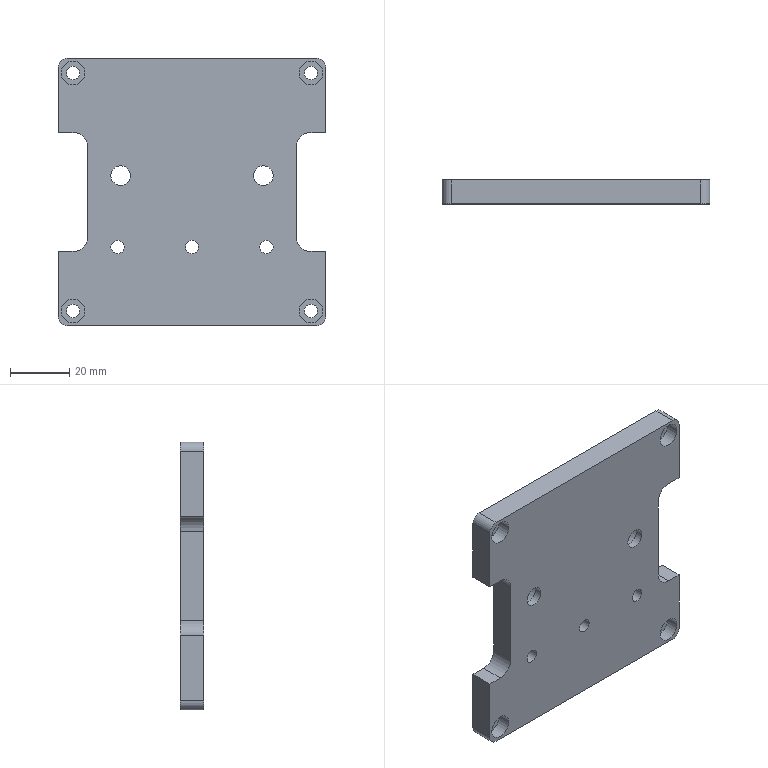Part | NX | 1 solid | 53 faces | box 90 x 8 x 90 mm | volume 55259 mm3 | cylinder 28 | plane 23 | cone 2 | commonest cylinder face diameters 4.5 x7 8 x7 6 x4 10 x4 2.5 x2 6.6 x2
STEP:
#1=CARTESIAN_POINT('',(45.,-4.,42.));
#2=VERTEX_POINT('',#1);
#3=CARTESIAN_POINT('',(45.,-4.,20.));
#4=VERTEX_POINT('',#3);
#5=CARTESIAN_POINT('',(45.,-4.,45.));
#6=DIRECTION('',(0.,0.,-1.));
#7=VECTOR('',#6,1000.);
#8=LINE('',#5,#7);
#9=EDGE_CURVE('',#2,#4,#8,.T.);
#10=ORIENTED_EDGE('',*,*,#9,.T.);
#11=CARTESIAN_POINT('',(45.,4.,20.));
#12=VERTEX_POINT('',#11);
#13=CARTESIAN_POINT('',(45.,4.,20.));
#14=DIRECTION('',(0.,1.,0.));
#15=VECTOR('',#14,1000.);
#16=LINE('',#13,#15);
#17=EDGE_CURVE('',#4,#12,#16,.T.);
#18=ORIENTED_EDGE('',*,*,#17,.T.);
#19=CARTESIAN_POINT('',(45.,4.,42.));
#20=VERTEX_POINT('',#19);
#21=CARTESIAN_POINT('',(45.,4.,45.));
#22=DIRECTION('',(0.,0.,-1.));
#23=VECTOR('',#22,1000.);
#24=LINE('',#21,#23);
#25=EDGE_CURVE('',#20,#12,#24,.T.);
#26=ORIENTED_EDGE('',*,*,#25,.F.);
#27=CARTESIAN_POINT('',(45.,4.,42.));
#28=DIRECTION('',(0.,-1.,0.));
#29=VECTOR('',#28,1000.);
#30=LINE('',#27,#29);
#31=EDGE_CURVE('',#20,#2,#30,.T.);
#32=ORIENTED_EDGE('',*,*,#31,.T.);
#33=EDGE_LOOP('',(#10,#18,#26,#32));
#34=FACE_BOUND('',#33,.T.);
#35=CARTESIAN_POINT('',(45.,4.,45.));
#36=DIRECTION('',(-1.,0.,0.));
#37=DIRECTION('',(0.,0.,1.));
#38=AXIS2_PLACEMENT_3D('',#35,#36,#37);
#39=PLANE('',#38);
#40=ADVANCED_FACE('',(#34),#39,.F.);
#41=CARTESIAN_POINT('',(-45.,4.,20.));
#42=VERTEX_POINT('',#41);
#43=CARTESIAN_POINT('',(-45.,4.,42.));
#44=VERTEX_POINT('',#43);
#45=CARTESIAN_POINT('',(-45.,4.,45.));
#46=DIRECTION('',(0.,0.,1.));
#47=VECTOR('',#46,1000.);
#48=LINE('',#45,#47);
#49=EDGE_CURVE('',#42,#44,#48,.T.);
#50=ORIENTED_EDGE('',*,*,#49,.F.);
#51=CARTESIAN_POINT('',(-45.,-4.,20.));
#52=VERTEX_POINT('',#51);
#53=CARTESIAN_POINT('',(-45.,4.,20.));
#54=DIRECTION('',(0.,-1.,0.));
#55=VECTOR('',#54,1000.);
#56=LINE('',#53,#55);
#57=EDGE_CURVE('',#42,#52,#56,.T.);
#58=ORIENTED_EDGE('',*,*,#57,.T.);
#59=CARTESIAN_POINT('',(-45.,-4.,42.));
#60=VERTEX_POINT('',#59);
#61=CARTESIAN_POINT('',(-45.,-4.,45.));
#62=DIRECTION('',(0.,0.,1.));
#63=VECTOR('',#62,1000.);
#64=LINE('',#61,#63);
#65=EDGE_CURVE('',#52,#60,#64,.T.);
#66=ORIENTED_EDGE('',*,*,#65,.T.);
#67=CARTESIAN_POINT('',(-45.,4.,42.));
#68=DIRECTION('',(0.,-1.,0.));
#69=VECTOR('',#68,1000.);
#70=LINE('',#67,#69);
#71=EDGE_CURVE('',#60,#44,#70,.F.);
#72=ORIENTED_EDGE('',*,*,#71,.T.);
#73=EDGE_LOOP('',(#50,#58,#66,#72));
#74=FACE_BOUND('',#73,.T.);
#75=CARTESIAN_POINT('',(-45.,4.,45.));
#76=DIRECTION('',(1.,0.,0.));
#77=DIRECTION('',(0.,0.,-1.));
#78=AXIS2_PLACEMENT_3D('',#75,#76,#77);
#79=PLANE('',#78);
#80=ADVANCED_FACE('',(#74),#79,.F.);
#81=CARTESIAN_POINT('',(-45.,-4.,-42.));
#82=VERTEX_POINT('',#81);
#83=CARTESIAN_POINT('',(-45.,-4.,-20.));
#84=VERTEX_POINT('',#83);
#85=CARTESIAN_POINT('',(-45.,-4.,45.));
#86=DIRECTION('',(0.,0.,1.));
#87=VECTOR('',#86,1000.);
#88=LINE('',#85,#87);
#89=EDGE_CURVE('',#82,#84,#88,.T.);
#90=ORIENTED_EDGE('',*,*,#89,.T.);
#91=CARTESIAN_POINT('',(-45.,4.,-20.));
#92=VERTEX_POINT('',#91);
#93=CARTESIAN_POINT('',(-45.,4.,-20.));
#94=DIRECTION('',(0.,1.,0.));
#95=VECTOR('',#94,1000.);
#96=LINE('',#93,#95);
#97=EDGE_CURVE('',#84,#92,#96,.T.);
#98=ORIENTED_EDGE('',*,*,#97,.T.);
#99=CARTESIAN_POINT('',(-45.,4.,-42.));
#100=VERTEX_POINT('',#99);
#101=CARTESIAN_POINT('',(-45.,4.,45.));
#102=DIRECTION('',(0.,0.,1.));
#103=VECTOR('',#102,1000.);
#104=LINE('',#101,#103);
#105=EDGE_CURVE('',#100,#92,#104,.T.);
#106=ORIENTED_EDGE('',*,*,#105,.F.);
#107=CARTESIAN_POINT('',(-45.,4.,-42.));
#108=DIRECTION('',(0.,-1.,0.));
#109=VECTOR('',#108,1000.);
#110=LINE('',#107,#109);
#111=EDGE_CURVE('',#100,#82,#110,.T.);
#112=ORIENTED_EDGE('',*,*,#111,.T.);
#113=EDGE_LOOP('',(#90,#98,#106,#112));
#114=FACE_BOUND('',#113,.T.);
#115=CARTESIAN_POINT('',(-45.,4.,45.));
#116=DIRECTION('',(1.,0.,0.));
#117=DIRECTION('',(0.,0.,-1.));
#118=AXIS2_PLACEMENT_3D('',#115,#116,#117);
#119=PLANE('',#118);
#120=ADVANCED_FACE('',(#114),#119,.F.);
#121=CARTESIAN_POINT('',(-42.,-4.,45.));
#122=VERTEX_POINT('',#121);
#123=CARTESIAN_POINT('',(42.,-4.,45.));
#124=VERTEX_POINT('',#123);
#125=CARTESIAN_POINT('',(45.,-4.,45.));
#126=DIRECTION('',(1.,0.,0.));
#127=VECTOR('',#126,1000.);
#128=LINE('',#125,#127);
#129=EDGE_CURVE('',#122,#124,#128,.T.);
#130=ORIENTED_EDGE('',*,*,#129,.T.);
#131=CARTESIAN_POINT('',(42.,4.,45.));
#132=VERTEX_POINT('',#131);
#133=CARTESIAN_POINT('',(42.,4.,45.));
#134=DIRECTION('',(0.,-1.,0.));
#135=VECTOR('',#134,1000.);
#136=LINE('',#133,#135);
#137=EDGE_CURVE('',#124,#132,#136,.F.);
#138=ORIENTED_EDGE('',*,*,#137,.T.);
#139=CARTESIAN_POINT('',(-42.,4.,45.));
#140=VERTEX_POINT('',#139);
#141=CARTESIAN_POINT('',(45.,4.,45.));
#142=DIRECTION('',(1.,0.,0.));
#143=VECTOR('',#142,1000.);
#144=LINE('',#141,#143);
#145=EDGE_CURVE('',#140,#132,#144,.T.);
#146=ORIENTED_EDGE('',*,*,#145,.F.);
#147=CARTESIAN_POINT('',(-42.,4.,45.));
#148=DIRECTION('',(0.,-1.,0.));
#149=VECTOR('',#148,1000.);
#150=LINE('',#147,#149);
#151=EDGE_CURVE('',#140,#122,#150,.T.);
#152=ORIENTED_EDGE('',*,*,#151,.T.);
#153=EDGE_LOOP('',(#130,#138,#146,#152));
#154=FACE_BOUND('',#153,.T.);
#155=CARTESIAN_POINT('',(45.,4.,45.));
#156=DIRECTION('',(0.,0.,-1.));
#157=DIRECTION('',(-1.,0.,0.));
#158=AXIS2_PLACEMENT_3D('',#155,#156,#157);
#159=PLANE('',#158);
#160=ADVANCED_FACE('',(#154),#159,.F.);
#161=CARTESIAN_POINT('',(45.,4.,-20.));
#162=VERTEX_POINT('',#161);
#163=CARTESIAN_POINT('',(45.,4.,-42.));
#164=VERTEX_POINT('',#163);
#165=CARTESIAN_POINT('',(45.,4.,45.));
#166=DIRECTION('',(0.,0.,-1.));
#167=VECTOR('',#166,1000.);
#168=LINE('',#165,#167);
#169=EDGE_CURVE('',#162,#164,#168,.T.);
#170=ORIENTED_EDGE('',*,*,#169,.F.);
#171=CARTESIAN_POINT('',(45.,-4.,-20.));
#172=VERTEX_POINT('',#171);
#173=CARTESIAN_POINT('',(45.,4.,-20.));
#174=DIRECTION('',(0.,-1.,0.));
#175=VECTOR('',#174,1000.);
#176=LINE('',#173,#175);
#177=EDGE_CURVE('',#162,#172,#176,.T.);
#178=ORIENTED_EDGE('',*,*,#177,.T.);
#179=CARTESIAN_POINT('',(45.,-4.,-42.));
#180=VERTEX_POINT('',#179);
#181=CARTESIAN_POINT('',(45.,-4.,45.));
#182=DIRECTION('',(0.,0.,-1.));
#183=VECTOR('',#182,1000.);
#184=LINE('',#181,#183);
#185=EDGE_CURVE('',#172,#180,#184,.T.);
#186=ORIENTED_EDGE('',*,*,#185,.T.);
#187=CARTESIAN_POINT('',(45.,4.,-42.));
#188=DIRECTION('',(0.,-1.,0.));
#189=VECTOR('',#188,1000.);
#190=LINE('',#187,#189);
#191=EDGE_CURVE('',#180,#164,#190,.F.);
#192=ORIENTED_EDGE('',*,*,#191,.T.);
#193=EDGE_LOOP('',(#170,#178,#186,#192));
#194=FACE_BOUND('',#193,.T.);
#195=CARTESIAN_POINT('',(45.,4.,45.));
#196=DIRECTION('',(-1.,0.,0.));
#197=DIRECTION('',(0.,0.,1.));
#198=AXIS2_PLACEMENT_3D('',#195,#196,#197);
#199=PLANE('',#198);
#200=ADVANCED_FACE('',(#194),#199,.F.);
#201=CARTESIAN_POINT('',(-13.75,0.,-45.));
#202=VERTEX_POINT('',#201);
#203=CARTESIAN_POINT('',(-12.5,0.,-45.));
#204=DIRECTION('',(0.,0.,-1.));
#205=DIRECTION('',(-1.,0.,0.));
#206=AXIS2_PLACEMENT_3D('',#203,#204,#205);
#207=CIRCLE('',#206,1.25);
#208=EDGE_CURVE('',#202,#202,#207,.T.);
#209=ORIENTED_EDGE('',*,*,#208,.F.);
#210=EDGE_LOOP('',(#209));
#211=FACE_BOUND('',#210,.T.);
#212=CARTESIAN_POINT('',(11.25,0.,-45.));
#213=VERTEX_POINT('',#212);
#214=CARTESIAN_POINT('',(12.5,0.,-45.));
#215=DIRECTION('',(0.,0.,-1.));
#216=DIRECTION('',(-1.,0.,0.));
#217=AXIS2_PLACEMENT_3D('',#214,#215,#216);
#218=CIRCLE('',#217,1.25);
#219=EDGE_CURVE('',#213,#213,#218,.T.);
#220=ORIENTED_EDGE('',*,*,#219,.F.);
#221=EDGE_LOOP('',(#220));
#222=FACE_BOUND('',#221,.T.);
#223=CARTESIAN_POINT('',(42.,-4.,-45.));
#224=VERTEX_POINT('',#223);
#225=CARTESIAN_POINT('',(-42.,-4.,-45.));
#226=VERTEX_POINT('',#225);
#227=CARTESIAN_POINT('',(45.,-4.,-45.));
#228=DIRECTION('',(-1.,0.,0.));
#229=VECTOR('',#228,1000.);
#230=LINE('',#227,#229);
#231=EDGE_CURVE('',#224,#226,#230,.T.);
#232=ORIENTED_EDGE('',*,*,#231,.T.);
#233=CARTESIAN_POINT('',(-42.,4.,-45.));
#234=VERTEX_POINT('',#233);
#235=CARTESIAN_POINT('',(-42.,4.,-45.));
#236=DIRECTION('',(0.,-1.,0.));
#237=VECTOR('',#236,1000.);
#238=LINE('',#235,#237);
#239=EDGE_CURVE('',#226,#234,#238,.F.);
#240=ORIENTED_EDGE('',*,*,#239,.T.);
#241=CARTESIAN_POINT('',(42.,4.,-45.));
#242=VERTEX_POINT('',#241);
#243=CARTESIAN_POINT('',(45.,4.,-45.));
#244=DIRECTION('',(-1.,0.,0.));
#245=VECTOR('',#244,1000.);
#246=LINE('',#243,#245);
#247=EDGE_CURVE('',#242,#234,#246,.T.);
#248=ORIENTED_EDGE('',*,*,#247,.F.);
#249=CARTESIAN_POINT('',(42.,4.,-45.));
#250=DIRECTION('',(0.,-1.,0.));
#251=VECTOR('',#250,1000.);
#252=LINE('',#249,#251);
#253=EDGE_CURVE('',#242,#224,#252,.T.);
#254=ORIENTED_EDGE('',*,*,#253,.T.);
#255=EDGE_LOOP('',(#232,#240,#248,#254));
#256=FACE_BOUND('',#255,.T.);
#257=CARTESIAN_POINT('',(45.,4.,-45.));
#258=DIRECTION('',(0.,0.,1.));
#259=DIRECTION('',(1.,0.,0.));
#260=AXIS2_PLACEMENT_3D('',#257,#258,#259);
#261=PLANE('',#260);
#262=ADVANCED_FACE('',(#211,#222,#256),#261,.F.);
#263=CARTESIAN_POINT('',(40.,4.,20.));
#264=VERTEX_POINT('',#263);
#265=CARTESIAN_POINT('',(35.,4.,20.));
#266=DIRECTION('',(-1.,0.,0.));
#267=VECTOR('',#266,1000.);
#268=LINE('',#265,#267);
#269=EDGE_CURVE('',#12,#264,#268,.T.);
#270=ORIENTED_EDGE('',*,*,#269,.T.);
#271=CARTESIAN_POINT('',(35.,4.,15.));
#272=VERTEX_POINT('',#271);
#273=CARTESIAN_POINT('',(40.,4.,15.));
#274=DIRECTION('',(0.,1.,0.));
#275=DIRECTION('',(0.,0.,1.));
#276=AXIS2_PLACEMENT_3D('',#273,#274,#275);
#277=CIRCLE('',#276,5.);
#278=EDGE_CURVE('',#264,#272,#277,.F.);
#279=ORIENTED_EDGE('',*,*,#278,.T.);
#280=CARTESIAN_POINT('',(35.,4.,-15.));
#281=VERTEX_POINT('',#280);
#282=CARTESIAN_POINT('',(35.,4.,20.));
#283=DIRECTION('',(0.,0.,-1.));
#284=VECTOR('',#283,1000.);
#285=LINE('',#282,#284);
#286=EDGE_CURVE('',#272,#281,#285,.T.);
#287=ORIENTED_EDGE('',*,*,#286,.T.);
#288=CARTESIAN_POINT('',(40.,4.,-20.));
#289=VERTEX_POINT('',#288);
#290=CARTESIAN_POINT('',(40.,4.,-15.));
#291=DIRECTION('',(0.,1.,0.));
#292=DIRECTION('',(0.,0.,1.));
#293=AXIS2_PLACEMENT_3D('',#290,#291,#292);
#294=CIRCLE('',#293,5.);
#295=EDGE_CURVE('',#281,#289,#294,.F.);
#296=ORIENTED_EDGE('',*,*,#295,.T.);
#297=CARTESIAN_POINT('',(35.,4.,-20.));
#298=DIRECTION('',(1.,0.,0.));
#299=VECTOR('',#298,1000.);
#300=LINE('',#297,#299);
#301=EDGE_CURVE('',#289,#162,#300,.T.);
#302=ORIENTED_EDGE('',*,*,#301,.T.);
#303=ORIENTED_EDGE('',*,*,#169,.T.);
#304=CARTESIAN_POINT('',(42.,4.,-42.));
#305=DIRECTION('',(0.,1.,0.));
#306=DIRECTION('',(0.,0.,1.));
#307=AXIS2_PLACEMENT_3D('',#304,#305,#306);
#308=CIRCLE('',#307,3.);
#309=EDGE_CURVE('',#164,#242,#308,.T.);
#310=ORIENTED_EDGE('',*,*,#309,.T.);
#311=ORIENTED_EDGE('',*,*,#247,.T.);
#312=CARTESIAN_POINT('',(-42.,4.,-42.));
#313=DIRECTION('',(0.,1.,0.));
#314=DIRECTION('',(0.,0.,1.));
#315=AXIS2_PLACEMENT_3D('',#312,#313,#314);
#316=CIRCLE('',#315,3.);
#317=EDGE_CURVE('',#234,#100,#316,.T.);
#318=ORIENTED_EDGE('',*,*,#317,.T.);
#319=ORIENTED_EDGE('',*,*,#105,.T.);
#320=CARTESIAN_POINT('',(-40.,4.,-20.));
#321=VERTEX_POINT('',#320);
#322=CARTESIAN_POINT('',(-35.,4.,-20.));
#323=DIRECTION('',(1.,0.,0.));
#324=VECTOR('',#323,1000.);
#325=LINE('',#322,#324);
#326=EDGE_CURVE('',#92,#321,#325,.T.);
#327=ORIENTED_EDGE('',*,*,#326,.T.);
#328=CARTESIAN_POINT('',(-35.,4.,-15.));
#329=VERTEX_POINT('',#328);
#330=CARTESIAN_POINT('',(-40.,4.,-15.));
#331=DIRECTION('',(0.,1.,0.));
#332=DIRECTION('',(0.,0.,1.));
#333=AXIS2_PLACEMENT_3D('',#330,#331,#332);
#334=CIRCLE('',#333,5.);
#335=EDGE_CURVE('',#321,#329,#334,.F.);
#336=ORIENTED_EDGE('',*,*,#335,.T.);
#337=CARTESIAN_POINT('',(-35.,4.,15.));
#338=VERTEX_POINT('',#337);
#339=CARTESIAN_POINT('',(-35.,4.,20.));
#340=DIRECTION('',(0.,0.,1.));
#341=VECTOR('',#340,1000.);
#342=LINE('',#339,#341);
#343=EDGE_CURVE('',#329,#338,#342,.T.);
#344=ORIENTED_EDGE('',*,*,#343,.T.);
#345=CARTESIAN_POINT('',(-40.,4.,20.));
#346=VERTEX_POINT('',#345);
#347=CARTESIAN_POINT('',(-40.,4.,15.));
#348=DIRECTION('',(0.,1.,0.));
#349=DIRECTION('',(0.,0.,1.));
#350=AXIS2_PLACEMENT_3D('',#347,#348,#349);
#351=CIRCLE('',#350,5.);
#352=EDGE_CURVE('',#338,#346,#351,.F.);
#353=ORIENTED_EDGE('',*,*,#352,.T.);
#354=CARTESIAN_POINT('',(-35.,4.,20.));
#355=DIRECTION('',(-1.,0.,0.));
#356=VECTOR('',#355,1000.);
#357=LINE('',#354,#356);
#358=EDGE_CURVE('',#346,#42,#357,.T.);
#359=ORIENTED_EDGE('',*,*,#358,.T.);
#360=ORIENTED_EDGE('',*,*,#49,.T.);
#361=CARTESIAN_POINT('',(-42.,4.,42.));
#362=DIRECTION('',(0.,1.,0.));
#363=DIRECTION('',(0.,0.,1.));
#364=AXIS2_PLACEMENT_3D('',#361,#362,#363);
#365=CIRCLE('',#364,3.);
#366=EDGE_CURVE('',#44,#140,#365,.T.);
#367=ORIENTED_EDGE('',*,*,#366,.T.);
#368=ORIENTED_EDGE('',*,*,#145,.T.);
#369=CARTESIAN_POINT('',(42.,4.,42.));
#370=DIRECTION('',(0.,1.,0.));
#371=DIRECTION('',(0.,0.,1.));
#372=AXIS2_PLACEMENT_3D('',#369,#370,#371);
#373=CIRCLE('',#372,3.);
#374=EDGE_CURVE('',#132,#20,#373,.T.);
#375=ORIENTED_EDGE('',*,*,#374,.T.);
#376=ORIENTED_EDGE('',*,*,#25,.T.);
#377=EDGE_LOOP('',(#270,#279,#287,#296,#302,#303,#310,#311,#318,#319,#327,#336,#344,#353,#359,#360,#367,#368,#375,#376));
#378=FACE_BOUND('',#377,.T.);
#379=CARTESIAN_POINT('',(-25.,4.,-14.5));
#380=VERTEX_POINT('',#379);
#381=CARTESIAN_POINT('',(-25.,4.,-18.5));
#382=DIRECTION('',(0.,1.,0.));
#383=DIRECTION('',(0.,0.,1.));
#384=AXIS2_PLACEMENT_3D('',#381,#382,#383);
#385=CIRCLE('',#384,4.);
#386=EDGE_CURVE('',#380,#380,#385,.T.);
#387=ORIENTED_EDGE('',*,*,#386,.F.);
#388=EDGE_LOOP('',(#387));
#389=FACE_BOUND('',#388,.T.);
#390=CARTESIAN_POINT('',(0.,4.,-14.5));
#391=VERTEX_POINT('',#390);
#392=CARTESIAN_POINT('',(0.,4.,-18.5));
#393=DIRECTION('',(0.,1.,0.));
#394=DIRECTION('',(0.,0.,1.));
#395=AXIS2_PLACEMENT_3D('',#392,#393,#394);
#396=CIRCLE('',#395,4.);
#397=EDGE_CURVE('',#391,#391,#396,.T.);
#398=ORIENTED_EDGE('',*,*,#397,.F.);
#399=EDGE_LOOP('',(#398));
#400=FACE_BOUND('',#399,.T.);
#401=CARTESIAN_POINT('',(25.,4.,-14.5));
#402=VERTEX_POINT('',#401);
#403=CARTESIAN_POINT('',(25.,4.,-18.5));
#404=DIRECTION('',(0.,1.,0.));
#405=DIRECTION('',(0.,0.,1.));
#406=AXIS2_PLACEMENT_3D('',#403,#404,#405);
#407=CIRCLE('',#406,4.);
#408=EDGE_CURVE('',#402,#402,#407,.T.);
#409=ORIENTED_EDGE('',*,*,#408,.F.);
#410=EDGE_LOOP('',(#409));
#411=FACE_BOUND('',#410,.T.);
#412=CARTESIAN_POINT('',(24.,4.,11.));
#413=VERTEX_POINT('',#412);
#414=CARTESIAN_POINT('',(24.,4.,5.5));
#415=DIRECTION('',(0.,1.,0.));
#416=DIRECTION('',(0.,0.,1.));
#417=AXIS2_PLACEMENT_3D('',#414,#415,#416);
#418=CIRCLE('',#417,5.5);
#419=EDGE_CURVE('',#413,#413,#418,.T.);
#420=ORIENTED_EDGE('',*,*,#419,.F.);
#421=EDGE_LOOP('',(#420));
#422=FACE_BOUND('',#421,.T.);
#423=CARTESIAN_POINT('',(-24.,4.,11.));
#424=VERTEX_POINT('',#423);
#425=CARTESIAN_POINT('',(-24.,4.,5.5));
#426=DIRECTION('',(0.,1.,0.));
#427=DIRECTION('',(0.,0.,1.));
#428=AXIS2_PLACEMENT_3D('',#425,#426,#427);
#429=CIRCLE('',#428,5.5);
#430=EDGE_CURVE('',#424,#424,#429,.T.);
#431=ORIENTED_EDGE('',*,*,#430,.F.);
#432=EDGE_LOOP('',(#431));
#433=FACE_BOUND('',#432,.T.);
#434=CARTESIAN_POINT('',(-40.,4.,-42.25));
#435=VERTEX_POINT('',#434);
#436=CARTESIAN_POINT('',(-40.,4.,-40.));
#437=DIRECTION('',(0.,-1.,0.));
#438=DIRECTION('',(0.,0.,-1.));
#439=AXIS2_PLACEMENT_3D('',#436,#437,#438);
#440=CIRCLE('',#439,2.25);
#441=EDGE_CURVE('',#435,#435,#440,.T.);
#442=ORIENTED_EDGE('',*,*,#441,.T.);
#443=EDGE_LOOP('',(#442));
#444=FACE_BOUND('',#443,.T.);
#445=CARTESIAN_POINT('',(40.,4.,-42.25));
#446=VERTEX_POINT('',#445);
#447=CARTESIAN_POINT('',(40.,4.,-40.));
#448=DIRECTION('',(0.,-1.,0.));
#449=DIRECTION('',(0.,0.,-1.));
#450=AXIS2_PLACEMENT_3D('',#447,#448,#449);
#451=CIRCLE('',#450,2.25);
#452=EDGE_CURVE('',#446,#446,#451,.T.);
#453=ORIENTED_EDGE('',*,*,#452,.T.);
#454=EDGE_LOOP('',(#453));
#455=FACE_BOUND('',#454,.T.);
#456=CARTESIAN_POINT('',(-40.,4.,37.75));
#457=VERTEX_POINT('',#456);
#458=CARTESIAN_POINT('',(-40.,4.,40.));
#459=DIRECTION('',(0.,-1.,0.));
#460=DIRECTION('',(0.,0.,-1.));
#461=AXIS2_PLACEMENT_3D('',#458,#459,#460);
#462=CIRCLE('',#461,2.25);
#463=EDGE_CURVE('',#457,#457,#462,.T.);
#464=ORIENTED_EDGE('',*,*,#463,.T.);
#465=EDGE_LOOP('',(#464));
#466=FACE_BOUND('',#465,.T.);
#467=CARTESIAN_POINT('',(40.,4.,37.75));
#468=VERTEX_POINT('',#467);
#469=CARTESIAN_POINT('',(40.,4.,40.));
#470=DIRECTION('',(0.,-1.,0.));
#471=DIRECTION('',(0.,0.,-1.));
#472=AXIS2_PLACEMENT_3D('',#469,#470,#471);
#473=CIRCLE('',#472,2.25);
#474=EDGE_CURVE('',#468,#468,#473,.T.);
#475=ORIENTED_EDGE('',*,*,#474,.T.);
#476=EDGE_LOOP('',(#475));
#477=FACE_BOUND('',#476,.T.);
#478=CARTESIAN_POINT('',(0.,4.,0.));
#479=DIRECTION('',(0.,1.,0.));
#480=DIRECTION('',(0.,0.,1.));
#481=AXIS2_PLACEMENT_3D('',#478,#479,#480);
#482=PLANE('',#481);
#483=ADVANCED_FACE('',(#378,#389,#400,#411,#422,#433,#444,#455,#466,#477),#482,.T.);
#484=CARTESIAN_POINT('',(-25.,-4.,-16.25));
#485=VERTEX_POINT('',#484);
#486=CARTESIAN_POINT('',(-25.,-4.,-18.5));
#487=DIRECTION('',(0.,1.,0.));
#488=DIRECTION('',(0.,0.,1.));
#489=AXIS2_PLACEMENT_3D('',#486,#487,#488);
#490=CIRCLE('',#489,2.25);
#491=EDGE_CURVE('',#485,#485,#490,.T.);
#492=ORIENTED_EDGE('',*,*,#491,.T.);
#493=EDGE_LOOP('',(#492));
#494=FACE_BOUND('',#493,.T.);
#495=CARTESIAN_POINT('',(0.,-4.,-16.25));
#496=VERTEX_POINT('',#495);
#497=CARTESIAN_POINT('',(0.,-4.,-18.5));
#498=DIRECTION('',(0.,1.,0.));
#499=DIRECTION('',(0.,0.,1.));
#500=AXIS2_PLACEMENT_3D('',#497,#498,#499);
#501=CIRCLE('',#500,2.25);
#502=EDGE_CURVE('',#496,#496,#501,.T.);
#503=ORIENTED_EDGE('',*,*,#502,.T.);
#504=EDGE_LOOP('',(#503));
#505=FACE_BOUND('',#504,.T.);
#506=CARTESIAN_POINT('',(25.,-4.,-16.25));
#507=VERTEX_POINT('',#506);
#508=CARTESIAN_POINT('',(25.,-4.,-18.5));
#509=DIRECTION('',(0.,1.,0.));
#510=DIRECTION('',(0.,0.,1.));
#511=AXIS2_PLACEMENT_3D('',#508,#509,#510);
#512=CIRCLE('',#511,2.25);
#513=EDGE_CURVE('',#507,#507,#512,.T.);
#514=ORIENTED_EDGE('',*,*,#513,.T.);
#515=EDGE_LOOP('',(#514));
#516=FACE_BOUND('',#515,.T.);
#517=CARTESIAN_POINT('',(24.,-4.,8.8));
#518=VERTEX_POINT('',#517);
#519=CARTESIAN_POINT('',(24.,-4.,5.5));
#520=DIRECTION('',(0.,1.,0.));
#521=DIRECTION('',(0.,0.,1.));
#522=AXIS2_PLACEMENT_3D('',#519,#520,#521);
#523=CIRCLE('',#522,3.3);
#524=EDGE_CURVE('',#518,#518,#523,.T.);
#525=ORIENTED_EDGE('',*,*,#524,.T.);
#526=EDGE_LOOP('',(#525));
#527=FACE_BOUND('',#526,.T.);
#528=CARTESIAN_POINT('',(-24.,-4.,8.8));
#529=VERTEX_POINT('',#528);
#530=CARTESIAN_POINT('',(-24.,-4.,5.5));
#531=DIRECTION('',(0.,1.,0.));
#532=DIRECTION('',(0.,0.,1.));
#533=AXIS2_PLACEMENT_3D('',#530,#531,#532);
#534=CIRCLE('',#533,3.3);
#535=EDGE_CURVE('',#529,#529,#534,.T.);
#536=ORIENTED_EDGE('',*,*,#535,.T.);
#537=EDGE_LOOP('',(#536));
#538=FACE_BOUND('',#537,.T.);
#539=CARTESIAN_POINT('',(-40.,-4.,-44.));
#540=VERTEX_POINT('',#539);
#541=CARTESIAN_POINT('',(-40.,-4.,-40.));
#542=DIRECTION('',(0.,-1.,0.));
#543=DIRECTION('',(0.,0.,-1.));
#544=AXIS2_PLACEMENT_3D('',#541,#542,#543);
#545=CIRCLE('',#544,4.);
#546=EDGE_CURVE('',#540,#540,#545,.T.);
#547=ORIENTED_EDGE('',*,*,#546,.F.);
#548=EDGE_LOOP('',(#547));
#549=FACE_BOUND('',#548,.T.);
#550=CARTESIAN_POINT('',(40.,-4.,-44.));
#551=VERTEX_POINT('',#550);
#552=CARTESIAN_POINT('',(40.,-4.,-40.));
#553=DIRECTION('',(0.,-1.,0.));
#554=DIRECTION('',(0.,0.,-1.));
#555=AXIS2_PLACEMENT_3D('',#552,#553,#554);
#556=CIRCLE('',#555,4.);
#557=EDGE_CURVE('',#551,#551,#556,.T.);
#558=ORIENTED_EDGE('',*,*,#557,.F.);
#559=EDGE_LOOP('',(#558));
#560=FACE_BOUND('',#559,.T.);
#561=CARTESIAN_POINT('',(-40.,-4.,36.));
#562=VERTEX_POINT('',#561);
#563=CARTESIAN_POINT('',(-40.,-4.,40.));
#564=DIRECTION('',(0.,-1.,0.));
#565=DIRECTION('',(0.,0.,-1.));
#566=AXIS2_PLACEMENT_3D('',#563,#564,#565);
#567=CIRCLE('',#566,4.);
#568=EDGE_CURVE('',#562,#562,#567,.T.);
#569=ORIENTED_EDGE('',*,*,#568,.F.);
#570=EDGE_LOOP('',(#569));
#571=FACE_BOUND('',#570,.T.);
#572=CARTESIAN_POINT('',(40.,-4.,36.));
#573=VERTEX_POINT('',#572);
#574=CARTESIAN_POINT('',(40.,-4.,40.));
#575=DIRECTION('',(0.,-1.,0.));
#576=DIRECTION('',(0.,0.,-1.));
#577=AXIS2_PLACEMENT_3D('',#574,#575,#576);
#578=CIRCLE('',#577,4.);
#579=EDGE_CURVE('',#573,#573,#578,.T.);
#580=ORIENTED_EDGE('',*,*,#579,.F.);
#581=EDGE_LOOP('',(#580));
#582=FACE_BOUND('',#581,.T.);
#583=CARTESIAN_POINT('',(35.,-4.,15.));
#584=VERTEX_POINT('',#583);
#585=CARTESIAN_POINT('',(35.,-4.,-15.));
#586=VERTEX_POINT('',#585);
#587=CARTESIAN_POINT('',(35.,-4.,20.));
#588=DIRECTION('',(0.,0.,-1.));
#589=VECTOR('',#588,1000.);
#590=LINE('',#587,#589);
#591=EDGE_CURVE('',#584,#586,#590,.T.);
#592=ORIENTED_EDGE('',*,*,#591,.F.);
#593=CARTESIAN_POINT('',(40.,-4.,20.));
#594=VERTEX_POINT('',#593);
#595=CARTESIAN_POINT('',(40.,-4.,15.));
#596=DIRECTION('',(0.,1.,0.));
#597=DIRECTION('',(0.,0.,1.));
#598=AXIS2_PLACEMENT_3D('',#595,#596,#597);
#599=CIRCLE('',#598,5.);
#600=EDGE_CURVE('',#584,#594,#599,.T.);
#601=ORIENTED_EDGE('',*,*,#600,.T.);
#602=CARTESIAN_POINT('',(0.,-4.,20.));
#603=DIRECTION('',(1.,0.,0.));
#604=VECTOR('',#603,1000.);
#605=LINE('',#602,#604);
#606=EDGE_CURVE('',#594,#4,#605,.T.);
#607=ORIENTED_EDGE('',*,*,#606,.T.);
#608=ORIENTED_EDGE('',*,*,#9,.F.);
#609=CARTESIAN_POINT('',(42.,-4.,42.));
#610=DIRECTION('',(0.,1.,0.));
#611=DIRECTION('',(0.,0.,1.));
#612=AXIS2_PLACEMENT_3D('',#609,#610,#611);
#613=CIRCLE('',#612,3.);
#614=EDGE_CURVE('',#2,#124,#613,.F.);
#615=ORIENTED_EDGE('',*,*,#614,.T.);
#616=ORIENTED_EDGE('',*,*,#129,.F.);
#617=CARTESIAN_POINT('',(-42.,-4.,42.));
#618=DIRECTION('',(0.,1.,0.));
#619=DIRECTION('',(0.,0.,1.));
#620=AXIS2_PLACEMENT_3D('',#617,#618,#619);
#621=CIRCLE('',#620,3.);
#622=EDGE_CURVE('',#122,#60,#621,.F.);
#623=ORIENTED_EDGE('',*,*,#622,.T.);
#624=ORIENTED_EDGE('',*,*,#65,.F.);
#625=CARTESIAN_POINT('',(-40.,-4.,20.));
#626=VERTEX_POINT('',#625);
#627=CARTESIAN_POINT('',(-35.,-4.,20.));
#628=DIRECTION('',(-1.,0.,0.));
#629=VECTOR('',#628,1000.);
#630=LINE('',#627,#629);
#631=EDGE_CURVE('',#626,#52,#630,.T.);
#632=ORIENTED_EDGE('',*,*,#631,.F.);
#633=CARTESIAN_POINT('',(-35.,-4.,15.));
#634=VERTEX_POINT('',#633);
#635=CARTESIAN_POINT('',(-40.,-4.,15.));
#636=DIRECTION('',(0.,1.,0.));
#637=DIRECTION('',(0.,0.,1.));
#638=AXIS2_PLACEMENT_3D('',#635,#636,#637);
#639=CIRCLE('',#638,5.);
#640=EDGE_CURVE('',#626,#634,#639,.T.);
#641=ORIENTED_EDGE('',*,*,#640,.T.);
#642=CARTESIAN_POINT('',(-35.,-4.,-15.));
#643=VERTEX_POINT('',#642);
#644=CARTESIAN_POINT('',(-35.,-4.,20.));
#645=DIRECTION('',(0.,0.,1.));
#646=VECTOR('',#645,1000.);
#647=LINE('',#644,#646);
#648=EDGE_CURVE('',#643,#634,#647,.T.);
#649=ORIENTED_EDGE('',*,*,#648,.F.);
#650=CARTESIAN_POINT('',(-40.,-4.,-20.));
#651=VERTEX_POINT('',#650);
#652=CARTESIAN_POINT('',(-40.,-4.,-15.));
#653=DIRECTION('',(0.,1.,0.));
#654=DIRECTION('',(0.,0.,1.));
#655=AXIS2_PLACEMENT_3D('',#652,#653,#654);
#656=CIRCLE('',#655,5.);
#657=EDGE_CURVE('',#643,#651,#656,.T.);
#658=ORIENTED_EDGE('',*,*,#657,.T.);
#659=CARTESIAN_POINT('',(0.,-4.,-20.));
#660=DIRECTION('',(-1.,0.,0.));
#661=VECTOR('',#660,1000.);
#662=LINE('',#659,#661);
#663=EDGE_CURVE('',#651,#84,#662,.T.);
#664=ORIENTED_EDGE('',*,*,#663,.T.);
#665=ORIENTED_EDGE('',*,*,#89,.F.);
#666=CARTESIAN_POINT('',(-42.,-4.,-42.));
#667=DIRECTION('',(0.,1.,0.));
#668=DIRECTION('',(0.,0.,1.));
#669=AXIS2_PLACEMENT_3D('',#666,#667,#668);
#670=CIRCLE('',#669,3.);
#671=EDGE_CURVE('',#82,#226,#670,.F.);
#672=ORIENTED_EDGE('',*,*,#671,.T.);
#673=ORIENTED_EDGE('',*,*,#231,.F.);
#674=CARTESIAN_POINT('',(42.,-4.,-42.));
#675=DIRECTION('',(0.,1.,0.));
#676=DIRECTION('',(0.,0.,1.));
#677=AXIS2_PLACEMENT_3D('',#674,#675,#676);
#678=CIRCLE('',#677,3.);
#679=EDGE_CURVE('',#224,#180,#678,.F.);
#680=ORIENTED_EDGE('',*,*,#679,.T.);
#681=ORIENTED_EDGE('',*,*,#185,.F.);
#682=CARTESIAN_POINT('',(40.,-4.,-20.));
#683=VERTEX_POINT('',#682);
#684=CARTESIAN_POINT('',(35.,-4.,-20.));
#685=DIRECTION('',(1.,0.,0.));
#686=VECTOR('',#685,1000.);
#687=LINE('',#684,#686);
#688=EDGE_CURVE('',#683,#172,#687,.T.);
#689=ORIENTED_EDGE('',*,*,#688,.F.);
#690=CARTESIAN_POINT('',(40.,-4.,-15.));
#691=DIRECTION('',(0.,1.,0.));
#692=DIRECTION('',(0.,0.,1.));
#693=AXIS2_PLACEMENT_3D('',#690,#691,#692);
#694=CIRCLE('',#693,5.);
#695=EDGE_CURVE('',#683,#586,#694,.T.);
#696=ORIENTED_EDGE('',*,*,#695,.T.);
#697=EDGE_LOOP('',(#592,#601,#607,#608,#615,#616,#623,#624,#632,#641,#649,#658,#664,#665,#672,#673,#680,#681,#689,#696));
#698=FACE_BOUND('',#697,.T.);
#699=CARTESIAN_POINT('',(0.,-4.,0.));
#700=DIRECTION('',(0.,1.,0.));
#701=DIRECTION('',(0.,0.,1.));
#702=AXIS2_PLACEMENT_3D('',#699,#700,#701);
#703=PLANE('',#702);
#704=ADVANCED_FACE('',(#494,#505,#516,#527,#538,#549,#560,#571,#582,#698),#703,.F.);
#705=ORIENTED_EDGE('',*,*,#474,.F.);
#706=EDGE_LOOP('',(#705));
#707=FACE_BOUND('',#706,.T.);
#708=CARTESIAN_POINT('',(40.,0.4,37.75));
#709=VERTEX_POINT('',#708);
#710=CARTESIAN_POINT('',(40.,0.4,40.));
#711=DIRECTION('',(0.,-1.,0.));
#712=DIRECTION('',(0.,0.,-1.));
#713=AXIS2_PLACEMENT_3D('',#710,#711,#712);
#714=CIRCLE('',#713,2.25);
#715=EDGE_CURVE('',#709,#709,#714,.T.);
#716=ORIENTED_EDGE('',*,*,#715,.T.);
#717=EDGE_LOOP('',(#716));
#718=FACE_BOUND('',#717,.T.);
#719=CARTESIAN_POINT('',(40.,-4.,40.));
#720=DIRECTION('',(0.,-1.,0.));
#721=DIRECTION('',(0.,0.,-1.));
#722=AXIS2_PLACEMENT_3D('',#719,#720,#721);
#723=CYLINDRICAL_SURFACE('',#722,2.25);
#724=ADVANCED_FACE('',(#707,#718),#723,.F.);
#725=ORIENTED_EDGE('',*,*,#715,.F.);
#726=EDGE_LOOP('',(#725));
#727=FACE_BOUND('',#726,.T.);
#728=CARTESIAN_POINT('',(40.,0.4,36.));
#729=VERTEX_POINT('',#728);
#730=CARTESIAN_POINT('',(40.,0.4,40.));
#731=DIRECTION('',(0.,-1.,0.));
#732=DIRECTION('',(0.,0.,-1.));
#733=AXIS2_PLACEMENT_3D('',#730,#731,#732);
#734=CIRCLE('',#733,4.);
#735=EDGE_CURVE('',#729,#729,#734,.T.);
#736=ORIENTED_EDGE('',*,*,#735,.T.);
#737=EDGE_LOOP('',(#736));
#738=FACE_BOUND('',#737,.T.);
#739=CARTESIAN_POINT('',(42.25,0.4,40.));
#740=DIRECTION('',(0.,1.,0.));
#741=DIRECTION('',(0.,0.,1.));
#742=AXIS2_PLACEMENT_3D('',#739,#740,#741);
#743=PLANE('',#742);
#744=ADVANCED_FACE('',(#727,#738),#743,.F.);
#745=ORIENTED_EDGE('',*,*,#735,.F.);
#746=EDGE_LOOP('',(#745));
#747=FACE_BOUND('',#746,.T.);
#748=ORIENTED_EDGE('',*,*,#579,.T.);
#749=EDGE_LOOP('',(#748));
#750=FACE_BOUND('',#749,.T.);
#751=CARTESIAN_POINT('',(40.,-4.,40.));
#752=DIRECTION('',(0.,-1.,0.));
#753=DIRECTION('',(0.,0.,-1.));
#754=AXIS2_PLACEMENT_3D('',#751,#752,#753);
#755=CYLINDRICAL_SURFACE('',#754,4.);
#756=ADVANCED_FACE('',(#747,#750),#755,.F.);
#757=ORIENTED_EDGE('',*,*,#463,.F.);
#758=EDGE_LOOP('',(#757));
#759=FACE_BOUND('',#758,.T.);
#760=CARTESIAN_POINT('',(-40.,0.4,37.75));
#761=VERTEX_POINT('',#760);
#762=CARTESIAN_POINT('',(-40.,0.4,40.));
#763=DIRECTION('',(0.,-1.,0.));
#764=DIRECTION('',(0.,0.,-1.));
#765=AXIS2_PLACEMENT_3D('',#762,#763,#764);
#766=CIRCLE('',#765,2.25);
#767=EDGE_CURVE('',#761,#761,#766,.T.);
#768=ORIENTED_EDGE('',*,*,#767,.T.);
#769=EDGE_LOOP('',(#768));
#770=FACE_BOUND('',#769,.T.);
#771=CARTESIAN_POINT('',(-40.,-4.,40.));
#772=DIRECTION('',(0.,-1.,0.));
#773=DIRECTION('',(0.,0.,-1.));
#774=AXIS2_PLACEMENT_3D('',#771,#772,#773);
#775=CYLINDRICAL_SURFACE('',#774,2.25);
#776=ADVANCED_FACE('',(#759,#770),#775,.F.);
#777=ORIENTED_EDGE('',*,*,#767,.F.);
#778=EDGE_LOOP('',(#777));
#779=FACE_BOUND('',#778,.T.);
#780=CARTESIAN_POINT('',(-40.,0.4,36.));
#781=VERTEX_POINT('',#780);
#782=CARTESIAN_POINT('',(-40.,0.4,40.));
#783=DIRECTION('',(0.,-1.,0.));
#784=DIRECTION('',(0.,0.,-1.));
#785=AXIS2_PLACEMENT_3D('',#782,#783,#784);
#786=CIRCLE('',#785,4.);
#787=EDGE_CURVE('',#781,#781,#786,.T.);
#788=ORIENTED_EDGE('',*,*,#787,.T.);
#789=EDGE_LOOP('',(#788));
#790=FACE_BOUND('',#789,.T.);
#791=CARTESIAN_POINT('',(-37.75,0.4,40.));
#792=DIRECTION('',(0.,1.,0.));
#793=DIRECTION('',(0.,0.,1.));
#794=AXIS2_PLACEMENT_3D('',#791,#792,#793);
#795=PLANE('',#794);
#796=ADVANCED_FACE('',(#779,#790),#795,.F.);
#797=ORIENTED_EDGE('',*,*,#787,.F.);
#798=EDGE_LOOP('',(#797));
#799=FACE_BOUND('',#798,.T.);
#800=ORIENTED_EDGE('',*,*,#568,.T.);
#801=EDGE_LOOP('',(#800));
#802=FACE_BOUND('',#801,.T.);
#803=CARTESIAN_POINT('',(-40.,-4.,40.));
#804=DIRECTION('',(0.,-1.,0.));
#805=DIRECTION('',(0.,0.,-1.));
#806=AXIS2_PLACEMENT_3D('',#803,#804,#805);
#807=CYLINDRICAL_SURFACE('',#806,4.);
#808=ADVANCED_FACE('',(#799,#802),#807,.F.);
#809=ORIENTED_EDGE('',*,*,#452,.F.);
#810=EDGE_LOOP('',(#809));
#811=FACE_BOUND('',#810,.T.);
#812=CARTESIAN_POINT('',(40.,0.4,-42.25));
#813=VERTEX_POINT('',#812);
#814=CARTESIAN_POINT('',(40.,0.4,-40.));
#815=DIRECTION('',(0.,-1.,0.));
#816=DIRECTION('',(0.,0.,-1.));
#817=AXIS2_PLACEMENT_3D('',#814,#815,#816);
#818=CIRCLE('',#817,2.25);
#819=EDGE_CURVE('',#813,#813,#818,.T.);
#820=ORIENTED_EDGE('',*,*,#819,.T.);
#821=EDGE_LOOP('',(#820));
#822=FACE_BOUND('',#821,.T.);
#823=CARTESIAN_POINT('',(40.,-4.,-40.));
#824=DIRECTION('',(0.,-1.,0.));
#825=DIRECTION('',(0.,0.,-1.));
#826=AXIS2_PLACEMENT_3D('',#823,#824,#825);
#827=CYLINDRICAL_SURFACE('',#826,2.25);
#828=ADVANCED_FACE('',(#811,#822),#827,.F.);
#829=ORIENTED_EDGE('',*,*,#819,.F.);
#830=EDGE_LOOP('',(#829));
#831=FACE_BOUND('',#830,.T.);
#832=CARTESIAN_POINT('',(40.,0.4,-44.));
#833=VERTEX_POINT('',#832);
#834=CARTESIAN_POINT('',(40.,0.4,-40.));
#835=DIRECTION('',(0.,-1.,0.));
#836=DIRECTION('',(0.,0.,-1.));
#837=AXIS2_PLACEMENT_3D('',#834,#835,#836);
#838=CIRCLE('',#837,4.);
#839=EDGE_CURVE('',#833,#833,#838,.T.);
#840=ORIENTED_EDGE('',*,*,#839,.T.);
#841=EDGE_LOOP('',(#840));
#842=FACE_BOUND('',#841,.T.);
#843=CARTESIAN_POINT('',(42.25,0.4,-40.));
#844=DIRECTION('',(0.,1.,0.));
#845=DIRECTION('',(0.,0.,1.));
#846=AXIS2_PLACEMENT_3D('',#843,#844,#845);
#847=PLANE('',#846);
#848=ADVANCED_FACE('',(#831,#842),#847,.F.);
#849=ORIENTED_EDGE('',*,*,#839,.F.);
#850=EDGE_LOOP('',(#849));
#851=FACE_BOUND('',#850,.T.);
#852=ORIENTED_EDGE('',*,*,#557,.T.);
#853=EDGE_LOOP('',(#852));
#854=FACE_BOUND('',#853,.T.);
#855=CARTESIAN_POINT('',(40.,-4.,-40.));
#856=DIRECTION('',(0.,-1.,0.));
#857=DIRECTION('',(0.,0.,-1.));
#858=AXIS2_PLACEMENT_3D('',#855,#856,#857);
#859=CYLINDRICAL_SURFACE('',#858,4.);
#860=ADVANCED_FACE('',(#851,#854),#859,.F.);
#861=ORIENTED_EDGE('',*,*,#441,.F.);
#862=EDGE_LOOP('',(#861));
#863=FACE_BOUND('',#862,.T.);
#864=CARTESIAN_POINT('',(-40.,0.4,-42.25));
#865=VERTEX_POINT('',#864);
#866=CARTESIAN_POINT('',(-40.,0.4,-40.));
#867=DIRECTION('',(0.,-1.,0.));
#868=DIRECTION('',(0.,0.,-1.));
#869=AXIS2_PLACEMENT_3D('',#866,#867,#868);
#870=CIRCLE('',#869,2.25);
#871=EDGE_CURVE('',#865,#865,#870,.T.);
#872=ORIENTED_EDGE('',*,*,#871,.T.);
#873=EDGE_LOOP('',(#872));
#874=FACE_BOUND('',#873,.T.);
#875=CARTESIAN_POINT('',(-40.,-4.,-40.));
#876=DIRECTION('',(0.,-1.,0.));
#877=DIRECTION('',(0.,0.,-1.));
#878=AXIS2_PLACEMENT_3D('',#875,#876,#877);
#879=CYLINDRICAL_SURFACE('',#878,2.25);
#880=ADVANCED_FACE('',(#863,#874),#879,.F.);
#881=ORIENTED_EDGE('',*,*,#871,.F.);
#882=EDGE_LOOP('',(#881));
#883=FACE_BOUND('',#882,.T.);
#884=CARTESIAN_POINT('',(-40.,0.4,-44.));
#885=VERTEX_POINT('',#884);
#886=CARTESIAN_POINT('',(-40.,0.4,-40.));
#887=DIRECTION('',(0.,-1.,0.));
#888=DIRECTION('',(0.,0.,-1.));
#889=AXIS2_PLACEMENT_3D('',#886,#887,#888);
#890=CIRCLE('',#889,4.);
#891=EDGE_CURVE('',#885,#885,#890,.T.);
#892=ORIENTED_EDGE('',*,*,#891,.T.);
#893=EDGE_LOOP('',(#892));
#894=FACE_BOUND('',#893,.T.);
#895=CARTESIAN_POINT('',(-37.75,0.4,-40.));
#896=DIRECTION('',(0.,1.,0.));
#897=DIRECTION('',(0.,0.,1.));
#898=AXIS2_PLACEMENT_3D('',#895,#896,#897);
#899=PLANE('',#898);
#900=ADVANCED_FACE('',(#883,#894),#899,.F.);
#901=ORIENTED_EDGE('',*,*,#891,.F.);
#902=EDGE_LOOP('',(#901));
#903=FACE_BOUND('',#902,.T.);
#904=ORIENTED_EDGE('',*,*,#546,.T.);
#905=EDGE_LOOP('',(#904));
#906=FACE_BOUND('',#905,.T.);
#907=CARTESIAN_POINT('',(-40.,-4.,-40.));
#908=DIRECTION('',(0.,-1.,0.));
#909=DIRECTION('',(0.,0.,-1.));
#910=AXIS2_PLACEMENT_3D('',#907,#908,#909);
#911=CYLINDRICAL_SURFACE('',#910,4.);
#912=ADVANCED_FACE('',(#903,#906),#911,.F.);
#913=ORIENTED_EDGE('',*,*,#535,.F.);
#914=EDGE_LOOP('',(#913));
#915=FACE_BOUND('',#914,.T.);
#916=CARTESIAN_POINT('',(-24.,-1.5,8.8));
#917=VERTEX_POINT('',#916);
#918=CARTESIAN_POINT('',(-24.,-1.5,5.5));
#919=DIRECTION('',(0.,1.,0.));
#920=DIRECTION('',(0.,0.,1.));
#921=AXIS2_PLACEMENT_3D('',#918,#919,#920);
#922=CIRCLE('',#921,3.3);
#923=EDGE_CURVE('',#917,#917,#922,.T.);
#924=ORIENTED_EDGE('',*,*,#923,.T.);
#925=EDGE_LOOP('',(#924));
#926=FACE_BOUND('',#925,.T.);
#927=CARTESIAN_POINT('',(-24.,4.,5.5));
#928=DIRECTION('',(0.,1.,0.));
#929=DIRECTION('',(0.,0.,1.));
#930=AXIS2_PLACEMENT_3D('',#927,#928,#929);
#931=CYLINDRICAL_SURFACE('',#930,3.3);
#932=ADVANCED_FACE('',(#915,#926),#931,.F.);
#933=ORIENTED_EDGE('',*,*,#923,.F.);
#934=EDGE_LOOP('',(#933));
#935=FACE_BOUND('',#934,.T.);
#936=CARTESIAN_POINT('',(-24.,-1.5,11.));
#937=VERTEX_POINT('',#936);
#938=CARTESIAN_POINT('',(-24.,-1.5,5.5));
#939=DIRECTION('',(0.,1.,0.));
#940=DIRECTION('',(0.,0.,1.));
#941=AXIS2_PLACEMENT_3D('',#938,#939,#940);
#942=CIRCLE('',#941,5.5);
#943=EDGE_CURVE('',#937,#937,#942,.T.);
#944=ORIENTED_EDGE('',*,*,#943,.T.);
#945=EDGE_LOOP('',(#944));
#946=FACE_BOUND('',#945,.T.);
#947=CARTESIAN_POINT('',(-20.7,-1.5,5.5));
#948=DIRECTION('',(0.,-1.,0.));
#949=DIRECTION('',(0.,0.,-1.));
#950=AXIS2_PLACEMENT_3D('',#947,#948,#949);
#951=PLANE('',#950);
#952=ADVANCED_FACE('',(#935,#946),#951,.F.);
#953=ORIENTED_EDGE('',*,*,#943,.F.);
#954=EDGE_LOOP('',(#953));
#955=FACE_BOUND('',#954,.T.);
#956=ORIENTED_EDGE('',*,*,#430,.T.);
#957=EDGE_LOOP('',(#956));
#958=FACE_BOUND('',#957,.T.);
#959=CARTESIAN_POINT('',(-24.,4.,5.5));
#960=DIRECTION('',(0.,1.,0.));
#961=DIRECTION('',(0.,0.,1.));
#962=AXIS2_PLACEMENT_3D('',#959,#960,#961);
#963=CYLINDRICAL_SURFACE('',#962,5.5);
#964=ADVANCED_FACE('',(#955,#958),#963,.F.);
#965=ORIENTED_EDGE('',*,*,#524,.F.);
#966=EDGE_LOOP('',(#965));
#967=FACE_BOUND('',#966,.T.);
#968=CARTESIAN_POINT('',(24.,-1.5,8.8));
#969=VERTEX_POINT('',#968);
#970=CARTESIAN_POINT('',(24.,-1.5,5.5));
#971=DIRECTION('',(0.,1.,0.));
#972=DIRECTION('',(0.,0.,1.));
#973=AXIS2_PLACEMENT_3D('',#970,#971,#972);
#974=CIRCLE('',#973,3.3);
#975=EDGE_CURVE('',#969,#969,#974,.T.);
#976=ORIENTED_EDGE('',*,*,#975,.T.);
#977=EDGE_LOOP('',(#976));
#978=FACE_BOUND('',#977,.T.);
#979=CARTESIAN_POINT('',(24.,4.,5.5));
#980=DIRECTION('',(0.,1.,0.));
#981=DIRECTION('',(0.,0.,1.));
#982=AXIS2_PLACEMENT_3D('',#979,#980,#981);
#983=CYLINDRICAL_SURFACE('',#982,3.3);
#984=ADVANCED_FACE('',(#967,#978),#983,.F.);
#985=ORIENTED_EDGE('',*,*,#975,.F.);
#986=EDGE_LOOP('',(#985));
#987=FACE_BOUND('',#986,.T.);
#988=CARTESIAN_POINT('',(24.,-1.5,11.));
#989=VERTEX_POINT('',#988);
#990=CARTESIAN_POINT('',(24.,-1.5,5.5));
#991=DIRECTION('',(0.,1.,0.));
#992=DIRECTION('',(0.,0.,1.));
#993=AXIS2_PLACEMENT_3D('',#990,#991,#992);
#994=CIRCLE('',#993,5.5);
#995=EDGE_CURVE('',#989,#989,#994,.T.);
#996=ORIENTED_EDGE('',*,*,#995,.T.);
#997=EDGE_LOOP('',(#996));
#998=FACE_BOUND('',#997,.T.);
#999=CARTESIAN_POINT('',(27.3,-1.5,5.5));
#1000=DIRECTION('',(0.,-1.,0.));
#1001=DIRECTION('',(0.,0.,-1.));
#1002=AXIS2_PLACEMENT_3D('',#999,#1000,#1001);
#1003=PLANE('',#1002);
#1004=ADVANCED_FACE('',(#987,#998),#1003,.F.);
#1005=ORIENTED_EDGE('',*,*,#995,.F.);
#1006=EDGE_LOOP('',(#1005));
#1007=FACE_BOUND('',#1006,.T.);
#1008=ORIENTED_EDGE('',*,*,#419,.T.);
#1009=EDGE_LOOP('',(#1008));
#1010=FACE_BOUND('',#1009,.T.);
#1011=CARTESIAN_POINT('',(24.,4.,5.5));
#1012=DIRECTION('',(0.,1.,0.));
#1013=DIRECTION('',(0.,0.,1.));
#1014=AXIS2_PLACEMENT_3D('',#1011,#1012,#1013);
#1015=CYLINDRICAL_SURFACE('',#1014,5.5);
#1016=ADVANCED_FACE('',(#1007,#1010),#1015,.F.);
#1017=ORIENTED_EDGE('',*,*,#513,.F.);
#1018=EDGE_LOOP('',(#1017));
#1019=FACE_BOUND('',#1018,.T.);
#1020=CARTESIAN_POINT('',(25.,-0.4,-16.25));
#1021=VERTEX_POINT('',#1020);
#1022=CARTESIAN_POINT('',(25.,-0.4,-18.5));
#1023=DIRECTION('',(0.,1.,0.));
#1024=DIRECTION('',(0.,0.,1.));
#1025=AXIS2_PLACEMENT_3D('',#1022,#1023,#1024);
#1026=CIRCLE('',#1025,2.25);
#1027=EDGE_CURVE('',#1021,#1021,#1026,.T.);
#1028=ORIENTED_EDGE('',*,*,#1027,.T.);
#1029=EDGE_LOOP('',(#1028));
#1030=FACE_BOUND('',#1029,.T.);
#1031=CARTESIAN_POINT('',(25.,4.,-18.5));
#1032=DIRECTION('',(0.,1.,0.));
#1033=DIRECTION('',(0.,0.,1.));
#1034=AXIS2_PLACEMENT_3D('',#1031,#1032,#1033);
#1035=CYLINDRICAL_SURFACE('',#1034,2.25);
#1036=ADVANCED_FACE('',(#1019,#1030),#1035,.F.);
#1037=ORIENTED_EDGE('',*,*,#1027,.F.);
#1038=EDGE_LOOP('',(#1037));
#1039=FACE_BOUND('',#1038,.T.);
#1040=CARTESIAN_POINT('',(25.,-0.4,-14.5));
#1041=VERTEX_POINT('',#1040);
#1042=CARTESIAN_POINT('',(25.,-0.4,-18.5));
#1043=DIRECTION('',(0.,1.,0.));
#1044=DIRECTION('',(0.,0.,1.));
#1045=AXIS2_PLACEMENT_3D('',#1042,#1043,#1044);
#1046=CIRCLE('',#1045,4.);
#1047=EDGE_CURVE('',#1041,#1041,#1046,.T.);
#1048=ORIENTED_EDGE('',*,*,#1047,.T.);
#1049=EDGE_LOOP('',(#1048));
#1050=FACE_BOUND('',#1049,.T.);
#1051=CARTESIAN_POINT('',(27.25,-0.4,-18.5));
#1052=DIRECTION('',(0.,-1.,0.));
#1053=DIRECTION('',(0.,0.,-1.));
#1054=AXIS2_PLACEMENT_3D('',#1051,#1052,#1053);
#1055=PLANE('',#1054);
#1056=ADVANCED_FACE('',(#1039,#1050),#1055,.F.);
#1057=ORIENTED_EDGE('',*,*,#1047,.F.);
#1058=EDGE_LOOP('',(#1057));
#1059=FACE_BOUND('',#1058,.T.);
#1060=ORIENTED_EDGE('',*,*,#408,.T.);
#1061=EDGE_LOOP('',(#1060));
#1062=FACE_BOUND('',#1061,.T.);
#1063=CARTESIAN_POINT('',(25.,4.,-18.5));
#1064=DIRECTION('',(0.,1.,0.));
#1065=DIRECTION('',(0.,0.,1.));
#1066=AXIS2_PLACEMENT_3D('',#1063,#1064,#1065);
#1067=CYLINDRICAL_SURFACE('',#1066,4.);
#1068=ADVANCED_FACE('',(#1059,#1062),#1067,.F.);
#1069=ORIENTED_EDGE('',*,*,#502,.F.);
#1070=EDGE_LOOP('',(#1069));
#1071=FACE_BOUND('',#1070,.T.);
#1072=CARTESIAN_POINT('',(0.,-0.4,-16.25));
#1073=VERTEX_POINT('',#1072);
#1074=CARTESIAN_POINT('',(0.,-0.4,-18.5));
#1075=DIRECTION('',(0.,1.,0.));
#1076=DIRECTION('',(0.,0.,1.));
#1077=AXIS2_PLACEMENT_3D('',#1074,#1075,#1076);
#1078=CIRCLE('',#1077,2.25);
#1079=EDGE_CURVE('',#1073,#1073,#1078,.T.);
#1080=ORIENTED_EDGE('',*,*,#1079,.T.);
#1081=EDGE_LOOP('',(#1080));
#1082=FACE_BOUND('',#1081,.T.);
#1083=CARTESIAN_POINT('',(0.,4.,-18.5));
#1084=DIRECTION('',(0.,1.,0.));
#1085=DIRECTION('',(0.,0.,1.));
#1086=AXIS2_PLACEMENT_3D('',#1083,#1084,#1085);
#1087=CYLINDRICAL_SURFACE('',#1086,2.25);
#1088=ADVANCED_FACE('',(#1071,#1082),#1087,.F.);
#1089=ORIENTED_EDGE('',*,*,#1079,.F.);
#1090=EDGE_LOOP('',(#1089));
#1091=FACE_BOUND('',#1090,.T.);
#1092=CARTESIAN_POINT('',(0.,-0.4,-14.5));
#1093=VERTEX_POINT('',#1092);
#1094=CARTESIAN_POINT('',(0.,-0.4,-18.5));
#1095=DIRECTION('',(0.,1.,0.));
#1096=DIRECTION('',(0.,0.,1.));
#1097=AXIS2_PLACEMENT_3D('',#1094,#1095,#1096);
#1098=CIRCLE('',#1097,4.);
#1099=EDGE_CURVE('',#1093,#1093,#1098,.T.);
#1100=ORIENTED_EDGE('',*,*,#1099,.T.);
#1101=EDGE_LOOP('',(#1100));
#1102=FACE_BOUND('',#1101,.T.);
#1103=CARTESIAN_POINT('',(2.25,-0.4,-18.5));
#1104=DIRECTION('',(0.,-1.,0.));
#1105=DIRECTION('',(0.,0.,-1.));
#1106=AXIS2_PLACEMENT_3D('',#1103,#1104,#1105);
#1107=PLANE('',#1106);
#1108=ADVANCED_FACE('',(#1091,#1102),#1107,.F.);
#1109=ORIENTED_EDGE('',*,*,#1099,.F.);
#1110=EDGE_LOOP('',(#1109));
#1111=FACE_BOUND('',#1110,.T.);
#1112=ORIENTED_EDGE('',*,*,#397,.T.);
#1113=EDGE_LOOP('',(#1112));
#1114=FACE_BOUND('',#1113,.T.);
#1115=CARTESIAN_POINT('',(0.,4.,-18.5));
#1116=DIRECTION('',(0.,1.,0.));
#1117=DIRECTION('',(0.,0.,1.));
#1118=AXIS2_PLACEMENT_3D('',#1115,#1116,#1117);
#1119=CYLINDRICAL_SURFACE('',#1118,4.);
#1120=ADVANCED_FACE('',(#1111,#1114),#1119,.F.);
#1121=ORIENTED_EDGE('',*,*,#491,.F.);
#1122=EDGE_LOOP('',(#1121));
#1123=FACE_BOUND('',#1122,.T.);
#1124=CARTESIAN_POINT('',(-25.,-0.4,-16.25));
#1125=VERTEX_POINT('',#1124);
#1126=CARTESIAN_POINT('',(-25.,-0.4,-18.5));
#1127=DIRECTION('',(0.,1.,0.));
#1128=DIRECTION('',(0.,0.,1.));
#1129=AXIS2_PLACEMENT_3D('',#1126,#1127,#1128);
#1130=CIRCLE('',#1129,2.25);
#1131=EDGE_CURVE('',#1125,#1125,#1130,.T.);
#1132=ORIENTED_EDGE('',*,*,#1131,.T.);
#1133=EDGE_LOOP('',(#1132));
#1134=FACE_BOUND('',#1133,.T.);
#1135=CARTESIAN_POINT('',(-25.,4.,-18.5));
#1136=DIRECTION('',(0.,1.,0.));
#1137=DIRECTION('',(0.,0.,1.));
#1138=AXIS2_PLACEMENT_3D('',#1135,#1136,#1137);
#1139=CYLINDRICAL_SURFACE('',#1138,2.25);
#1140=ADVANCED_FACE('',(#1123,#1134),#1139,.F.);
#1141=ORIENTED_EDGE('',*,*,#1131,.F.);
#1142=EDGE_LOOP('',(#1141));
#1143=FACE_BOUND('',#1142,.T.);
#1144=CARTESIAN_POINT('',(-25.,-0.4,-14.5));
#1145=VERTEX_POINT('',#1144);
#1146=CARTESIAN_POINT('',(-25.,-0.4,-18.5));
#1147=DIRECTION('',(0.,1.,0.));
#1148=DIRECTION('',(0.,0.,1.));
#1149=AXIS2_PLACEMENT_3D('',#1146,#1147,#1148);
#1150=CIRCLE('',#1149,4.);
#1151=EDGE_CURVE('',#1145,#1145,#1150,.T.);
#1152=ORIENTED_EDGE('',*,*,#1151,.T.);
#1153=EDGE_LOOP('',(#1152));
#1154=FACE_BOUND('',#1153,.T.);
#1155=CARTESIAN_POINT('',(-22.75,-0.4,-18.5));
#1156=DIRECTION('',(0.,-1.,0.));
#1157=DIRECTION('',(0.,0.,-1.));
#1158=AXIS2_PLACEMENT_3D('',#1155,#1156,#1157);
#1159=PLANE('',#1158);
#1160=ADVANCED_FACE('',(#1143,#1154),#1159,.F.);
#1161=ORIENTED_EDGE('',*,*,#1151,.F.);
#1162=EDGE_LOOP('',(#1161));
#1163=FACE_BOUND('',#1162,.T.);
#1164=ORIENTED_EDGE('',*,*,#386,.T.);
#1165=EDGE_LOOP('',(#1164));
#1166=FACE_BOUND('',#1165,.T.);
#1167=CARTESIAN_POINT('',(-25.,4.,-18.5));
#1168=DIRECTION('',(0.,1.,0.));
#1169=DIRECTION('',(0.,0.,1.));
#1170=AXIS2_PLACEMENT_3D('',#1167,#1168,#1169);
#1171=CYLINDRICAL_SURFACE('',#1170,4.);
#1172=ADVANCED_FACE('',(#1163,#1166),#1171,.F.);
#1173=CARTESIAN_POINT('',(12.5,0.,-35.749));
#1174=VERTEX_POINT('',#1173);
#1175=VERTEX_LOOP('',#1174);
#1176=FACE_BOUND('',#1175,.T.);
#1177=CARTESIAN_POINT('',(11.25,0.,-36.5));
#1178=VERTEX_POINT('',#1177);
#1179=CARTESIAN_POINT('',(12.5,0.,-36.5));
#1180=DIRECTION('',(0.,0.,-1.));
#1181=DIRECTION('',(-1.,0.,0.));
#1182=AXIS2_PLACEMENT_3D('',#1179,#1180,#1181);
#1183=CIRCLE('',#1182,1.25);
#1184=EDGE_CURVE('',#1178,#1178,#1183,.T.);
#1185=ORIENTED_EDGE('',*,*,#1184,.T.);
#1186=EDGE_LOOP('',(#1185));
#1187=FACE_BOUND('',#1186,.T.);
#1188=CARTESIAN_POINT('',(12.5,0.,-36.5));
#1189=DIRECTION('',(0.,0.,-1.));
#1190=DIRECTION('',(-1.,0.,0.));
#1191=AXIS2_PLACEMENT_3D('',#1188,#1189,#1190);
#1192=CONICAL_SURFACE('',#1191,1.25,1.03);
#1193=ADVANCED_FACE('',(#1176,#1187),#1192,.F.);
#1194=ORIENTED_EDGE('',*,*,#1184,.F.);
#1195=EDGE_LOOP('',(#1194));
#1196=FACE_BOUND('',#1195,.T.);
#1197=ORIENTED_EDGE('',*,*,#219,.T.);
#1198=EDGE_LOOP('',(#1197));
#1199=FACE_BOUND('',#1198,.T.);
#1200=CARTESIAN_POINT('',(12.5,0.,-45.));
#1201=DIRECTION('',(0.,0.,-1.));
#1202=DIRECTION('',(-1.,0.,0.));
#1203=AXIS2_PLACEMENT_3D('',#1200,#1201,#1202);
#1204=CYLINDRICAL_SURFACE('',#1203,1.25);
#1205=ADVANCED_FACE('',(#1196,#1199),#1204,.F.);
#1206=CARTESIAN_POINT('',(-12.5,0.,-35.749));
#1207=VERTEX_POINT('',#1206);
#1208=VERTEX_LOOP('',#1207);
#1209=FACE_BOUND('',#1208,.T.);
#1210=CARTESIAN_POINT('',(-13.75,0.,-36.5));
#1211=VERTEX_POINT('',#1210);
#1212=CARTESIAN_POINT('',(-12.5,0.,-36.5));
#1213=DIRECTION('',(0.,0.,-1.));
#1214=DIRECTION('',(-1.,0.,0.));
#1215=AXIS2_PLACEMENT_3D('',#1212,#1213,#1214);
#1216=CIRCLE('',#1215,1.25);
#1217=EDGE_CURVE('',#1211,#1211,#1216,.T.);
#1218=ORIENTED_EDGE('',*,*,#1217,.T.);
#1219=EDGE_LOOP('',(#1218));
#1220=FACE_BOUND('',#1219,.T.);
#1221=CARTESIAN_POINT('',(-12.5,0.,-36.5));
#1222=DIRECTION('',(0.,0.,-1.));
#1223=DIRECTION('',(-1.,0.,0.));
#1224=AXIS2_PLACEMENT_3D('',#1221,#1222,#1223);
#1225=CONICAL_SURFACE('',#1224,1.25,1.03);
#1226=ADVANCED_FACE('',(#1209,#1220),#1225,.F.);
#1227=ORIENTED_EDGE('',*,*,#1217,.F.);
#1228=EDGE_LOOP('',(#1227));
#1229=FACE_BOUND('',#1228,.T.);
#1230=ORIENTED_EDGE('',*,*,#208,.T.);
#1231=EDGE_LOOP('',(#1230));
#1232=FACE_BOUND('',#1231,.T.);
#1233=CARTESIAN_POINT('',(-12.5,0.,-45.));
#1234=DIRECTION('',(0.,0.,-1.));
#1235=DIRECTION('',(-1.,0.,0.));
#1236=AXIS2_PLACEMENT_3D('',#1233,#1234,#1235);
#1237=CYLINDRICAL_SURFACE('',#1236,1.25);
#1238=ADVANCED_FACE('',(#1229,#1232),#1237,.F.);
#1239=ORIENTED_EDGE('',*,*,#317,.F.);
#1240=ORIENTED_EDGE('',*,*,#239,.F.);
#1241=ORIENTED_EDGE('',*,*,#671,.F.);
#1242=ORIENTED_EDGE('',*,*,#111,.F.);
#1243=EDGE_LOOP('',(#1239,#1240,#1241,#1242));
#1244=FACE_BOUND('',#1243,.T.);
#1245=CARTESIAN_POINT('',(-42.,4.,-42.));
#1246=DIRECTION('',(0.,-1.,0.));
#1247=DIRECTION('',(0.,0.,-1.));
#1248=AXIS2_PLACEMENT_3D('',#1245,#1246,#1247);
#1249=CYLINDRICAL_SURFACE('',#1248,3.);
#1250=ADVANCED_FACE('',(#1244),#1249,.T.);
#1251=ORIENTED_EDGE('',*,*,#309,.F.);
#1252=ORIENTED_EDGE('',*,*,#191,.F.);
#1253=ORIENTED_EDGE('',*,*,#679,.F.);
#1254=ORIENTED_EDGE('',*,*,#253,.F.);
#1255=EDGE_LOOP('',(#1251,#1252,#1253,#1254));
#1256=FACE_BOUND('',#1255,.T.);
#1257=CARTESIAN_POINT('',(42.,4.,-42.));
#1258=DIRECTION('',(0.,-1.,0.));
#1259=DIRECTION('',(0.,0.,-1.));
#1260=AXIS2_PLACEMENT_3D('',#1257,#1258,#1259);
#1261=CYLINDRICAL_SURFACE('',#1260,3.);
#1262=ADVANCED_FACE('',(#1256),#1261,.T.);
#1263=ORIENTED_EDGE('',*,*,#374,.F.);
#1264=ORIENTED_EDGE('',*,*,#137,.F.);
#1265=ORIENTED_EDGE('',*,*,#614,.F.);
#1266=ORIENTED_EDGE('',*,*,#31,.F.);
#1267=EDGE_LOOP('',(#1263,#1264,#1265,#1266));
#1268=FACE_BOUND('',#1267,.T.);
#1269=CARTESIAN_POINT('',(42.,4.,42.));
#1270=DIRECTION('',(0.,-1.,0.));
#1271=DIRECTION('',(0.,0.,-1.));
#1272=AXIS2_PLACEMENT_3D('',#1269,#1270,#1271);
#1273=CYLINDRICAL_SURFACE('',#1272,3.);
#1274=ADVANCED_FACE('',(#1268),#1273,.T.);
#1275=ORIENTED_EDGE('',*,*,#366,.F.);
#1276=ORIENTED_EDGE('',*,*,#71,.F.);
#1277=ORIENTED_EDGE('',*,*,#622,.F.);
#1278=ORIENTED_EDGE('',*,*,#151,.F.);
#1279=EDGE_LOOP('',(#1275,#1276,#1277,#1278));
#1280=FACE_BOUND('',#1279,.T.);
#1281=CARTESIAN_POINT('',(-42.,4.,42.));
#1282=DIRECTION('',(0.,-1.,0.));
#1283=DIRECTION('',(0.,0.,-1.));
#1284=AXIS2_PLACEMENT_3D('',#1281,#1282,#1283);
#1285=CYLINDRICAL_SURFACE('',#1284,3.);
#1286=ADVANCED_FACE('',(#1280),#1285,.T.);
#1287=ORIENTED_EDGE('',*,*,#358,.F.);
#1288=CARTESIAN_POINT('',(-40.,-4.,20.));
#1289=DIRECTION('',(0.,-1.,0.));
#1290=VECTOR('',#1289,1000.);
#1291=LINE('',#1288,#1290);
#1292=EDGE_CURVE('',#346,#626,#1291,.T.);
#1293=ORIENTED_EDGE('',*,*,#1292,.T.);
#1294=ORIENTED_EDGE('',*,*,#631,.T.);
#1295=ORIENTED_EDGE('',*,*,#57,.F.);
#1296=EDGE_LOOP('',(#1287,#1293,#1294,#1295));
#1297=FACE_BOUND('',#1296,.T.);
#1298=CARTESIAN_POINT('',(-35.,4.,20.));
#1299=DIRECTION('',(0.,0.,1.));
#1300=DIRECTION('',(1.,0.,0.));
#1301=AXIS2_PLACEMENT_3D('',#1298,#1299,#1300);
#1302=PLANE('',#1301);
#1303=ADVANCED_FACE('',(#1297),#1302,.F.);
#1304=ORIENTED_EDGE('',*,*,#663,.F.);
#1305=CARTESIAN_POINT('',(-40.,4.,-20.));
#1306=DIRECTION('',(0.,-1.,0.));
#1307=VECTOR('',#1306,1000.);
#1308=LINE('',#1305,#1307);
#1309=EDGE_CURVE('',#651,#321,#1308,.F.);
#1310=ORIENTED_EDGE('',*,*,#1309,.T.);
#1311=ORIENTED_EDGE('',*,*,#326,.F.);
#1312=ORIENTED_EDGE('',*,*,#97,.F.);
#1313=EDGE_LOOP('',(#1304,#1310,#1311,#1312));
#1314=FACE_BOUND('',#1313,.T.);
#1315=CARTESIAN_POINT('',(-35.,4.,-20.));
#1316=DIRECTION('',(0.,0.,-1.));
#1317=DIRECTION('',(-1.,0.,0.));
#1318=AXIS2_PLACEMENT_3D('',#1315,#1316,#1317);
#1319=PLANE('',#1318);
#1320=ADVANCED_FACE('',(#1314),#1319,.F.);
#1321=ORIENTED_EDGE('',*,*,#343,.F.);
#1322=CARTESIAN_POINT('',(-35.,-4.,-15.));
#1323=DIRECTION('',(0.,-1.,0.));
#1324=VECTOR('',#1323,1000.);
#1325=LINE('',#1322,#1324);
#1326=EDGE_CURVE('',#329,#643,#1325,.T.);
#1327=ORIENTED_EDGE('',*,*,#1326,.T.);
#1328=ORIENTED_EDGE('',*,*,#648,.T.);
#1329=CARTESIAN_POINT('',(-35.,4.,15.));
#1330=DIRECTION('',(0.,-1.,0.));
#1331=VECTOR('',#1330,1000.);
#1332=LINE('',#1329,#1331);
#1333=EDGE_CURVE('',#634,#338,#1332,.F.);
#1334=ORIENTED_EDGE('',*,*,#1333,.T.);
#1335=EDGE_LOOP('',(#1321,#1327,#1328,#1334));
#1336=FACE_BOUND('',#1335,.T.);
#1337=CARTESIAN_POINT('',(-35.,4.,20.));
#1338=DIRECTION('',(1.,0.,0.));
#1339=DIRECTION('',(0.,0.,-1.));
#1340=AXIS2_PLACEMENT_3D('',#1337,#1338,#1339);
#1341=PLANE('',#1340);
#1342=ADVANCED_FACE('',(#1336),#1341,.F.);
#1343=ORIENTED_EDGE('',*,*,#606,.F.);
#1344=CARTESIAN_POINT('',(40.,4.,20.));
#1345=DIRECTION('',(0.,-1.,0.));
#1346=VECTOR('',#1345,1000.);
#1347=LINE('',#1344,#1346);
#1348=EDGE_CURVE('',#594,#264,#1347,.F.);
#1349=ORIENTED_EDGE('',*,*,#1348,.T.);
#1350=ORIENTED_EDGE('',*,*,#269,.F.);
#1351=ORIENTED_EDGE('',*,*,#17,.F.);
#1352=EDGE_LOOP('',(#1343,#1349,#1350,#1351));
#1353=FACE_BOUND('',#1352,.T.);
#1354=CARTESIAN_POINT('',(35.,4.,20.));
#1355=DIRECTION('',(0.,0.,1.));
#1356=DIRECTION('',(1.,0.,0.));
#1357=AXIS2_PLACEMENT_3D('',#1354,#1355,#1356);
#1358=PLANE('',#1357);
#1359=ADVANCED_FACE('',(#1353),#1358,.F.);
#1360=ORIENTED_EDGE('',*,*,#301,.F.);
#1361=CARTESIAN_POINT('',(40.,-4.,-20.));
#1362=DIRECTION('',(0.,-1.,0.));
#1363=VECTOR('',#1362,1000.);
#1364=LINE('',#1361,#1363);
#1365=EDGE_CURVE('',#289,#683,#1364,.T.);
#1366=ORIENTED_EDGE('',*,*,#1365,.T.);
#1367=ORIENTED_EDGE('',*,*,#688,.T.);
#1368=ORIENTED_EDGE('',*,*,#177,.F.);
#1369=EDGE_LOOP('',(#1360,#1366,#1367,#1368));
#1370=FACE_BOUND('',#1369,.T.);
#1371=CARTESIAN_POINT('',(35.,4.,-20.));
#1372=DIRECTION('',(0.,0.,-1.));
#1373=DIRECTION('',(-1.,0.,0.));
#1374=AXIS2_PLACEMENT_3D('',#1371,#1372,#1373);
#1375=PLANE('',#1374);
#1376=ADVANCED_FACE('',(#1370),#1375,.F.);
#1377=ORIENTED_EDGE('',*,*,#591,.T.);
#1378=CARTESIAN_POINT('',(35.,4.,-15.));
#1379=DIRECTION('',(0.,-1.,0.));
#1380=VECTOR('',#1379,1000.);
#1381=LINE('',#1378,#1380);
#1382=EDGE_CURVE('',#586,#281,#1381,.F.);
#1383=ORIENTED_EDGE('',*,*,#1382,.T.);
#1384=ORIENTED_EDGE('',*,*,#286,.F.);
#1385=CARTESIAN_POINT('',(35.,-4.,15.));
#1386=DIRECTION('',(0.,-1.,0.));
#1387=VECTOR('',#1386,1000.);
#1388=LINE('',#1385,#1387);
#1389=EDGE_CURVE('',#272,#584,#1388,.T.);
#1390=ORIENTED_EDGE('',*,*,#1389,.T.);
#1391=EDGE_LOOP('',(#1377,#1383,#1384,#1390));
#1392=FACE_BOUND('',#1391,.T.);
#1393=CARTESIAN_POINT('',(35.,4.,20.));
#1394=DIRECTION('',(-1.,0.,0.));
#1395=DIRECTION('',(0.,0.,1.));
#1396=AXIS2_PLACEMENT_3D('',#1393,#1394,#1395);
#1397=PLANE('',#1396);
#1398=ADVANCED_FACE('',(#1392),#1397,.F.);
#1399=ORIENTED_EDGE('',*,*,#295,.F.);
#1400=ORIENTED_EDGE('',*,*,#1382,.F.);
#1401=ORIENTED_EDGE('',*,*,#695,.F.);
#1402=ORIENTED_EDGE('',*,*,#1365,.F.);
#1403=EDGE_LOOP('',(#1399,#1400,#1401,#1402));
#1404=FACE_BOUND('',#1403,.T.);
#1405=CARTESIAN_POINT('',(40.,4.,-15.));
#1406=DIRECTION('',(0.,1.,0.));
#1407=DIRECTION('',(0.,0.,1.));
#1408=AXIS2_PLACEMENT_3D('',#1405,#1406,#1407);
#1409=CYLINDRICAL_SURFACE('',#1408,5.);
#1410=ADVANCED_FACE('',(#1404),#1409,.F.);
#1411=ORIENTED_EDGE('',*,*,#278,.F.);
#1412=ORIENTED_EDGE('',*,*,#1348,.F.);
#1413=ORIENTED_EDGE('',*,*,#600,.F.);
#1414=ORIENTED_EDGE('',*,*,#1389,.F.);
#1415=EDGE_LOOP('',(#1411,#1412,#1413,#1414));
#1416=FACE_BOUND('',#1415,.T.);
#1417=CARTESIAN_POINT('',(40.,4.,15.));
#1418=DIRECTION('',(0.,1.,0.));
#1419=DIRECTION('',(0.,0.,1.));
#1420=AXIS2_PLACEMENT_3D('',#1417,#1418,#1419);
#1421=CYLINDRICAL_SURFACE('',#1420,5.);
#1422=ADVANCED_FACE('',(#1416),#1421,.F.);
#1423=ORIENTED_EDGE('',*,*,#335,.F.);
#1424=ORIENTED_EDGE('',*,*,#1309,.F.);
#1425=ORIENTED_EDGE('',*,*,#657,.F.);
#1426=ORIENTED_EDGE('',*,*,#1326,.F.);
#1427=EDGE_LOOP('',(#1423,#1424,#1425,#1426));
#1428=FACE_BOUND('',#1427,.T.);
#1429=CARTESIAN_POINT('',(-40.,4.,-15.));
#1430=DIRECTION('',(0.,1.,0.));
#1431=DIRECTION('',(0.,0.,1.));
#1432=AXIS2_PLACEMENT_3D('',#1429,#1430,#1431);
#1433=CYLINDRICAL_SURFACE('',#1432,5.);
#1434=ADVANCED_FACE('',(#1428),#1433,.F.);
#1435=ORIENTED_EDGE('',*,*,#352,.F.);
#1436=ORIENTED_EDGE('',*,*,#1333,.F.);
#1437=ORIENTED_EDGE('',*,*,#640,.F.);
#1438=ORIENTED_EDGE('',*,*,#1292,.F.);
#1439=EDGE_LOOP('',(#1435,#1436,#1437,#1438));
#1440=FACE_BOUND('',#1439,.T.);
#1441=CARTESIAN_POINT('',(-40.,4.,15.));
#1442=DIRECTION('',(0.,1.,0.));
#1443=DIRECTION('',(0.,0.,1.));
#1444=AXIS2_PLACEMENT_3D('',#1441,#1442,#1443);
#1445=CYLINDRICAL_SURFACE('',#1444,5.);
#1446=ADVANCED_FACE('',(#1440),#1445,.F.);
#1447=CLOSED_SHELL('',(#40,#80,#120,#160,#200,#262,#483,#704,#724,#744,#756,#776,#796,#808,#828,#848,#860,#880,#900,#912,#932,#952,#964,#984,#1004,#1016,#1036,#1056,#1068,#1088,#1108,#1120,#1140,#1160,#1172,#1193,#1205,#1226,#1238,#1250,#1262,#1274,#1286,#1303,#1320,#1342,#1359,#1376,#1398,#1410,#1422,#1434,#1446));
#1448=MANIFOLD_SOLID_BREP('',#1447);
#1449=(LENGTH_UNIT()NAMED_UNIT(*)SI_UNIT(.MILLI.,.METRE.));
#1450=UNCERTAINTY_MEASURE_WITH_UNIT(LENGTH_MEASURE(0.00001),#1449,'','');
#1451=(NAMED_UNIT(*)PLANE_ANGLE_UNIT()SI_UNIT($,.RADIAN.));
#1452=(NAMED_UNIT(*)SI_UNIT($,.STERADIAN.)SOLID_ANGLE_UNIT());
#1453=(GEOMETRIC_REPRESENTATION_CONTEXT(3)GLOBAL_UNCERTAINTY_ASSIGNED_CONTEXT((#1450))GLOBAL_UNIT_ASSIGNED_CONTEXT((#1449,#1451,#1452))REPRESENTATION_CONTEXT('',''));
#1454=ADVANCED_BREP_SHAPE_REPRESENTATION('',(#1448),#1453);